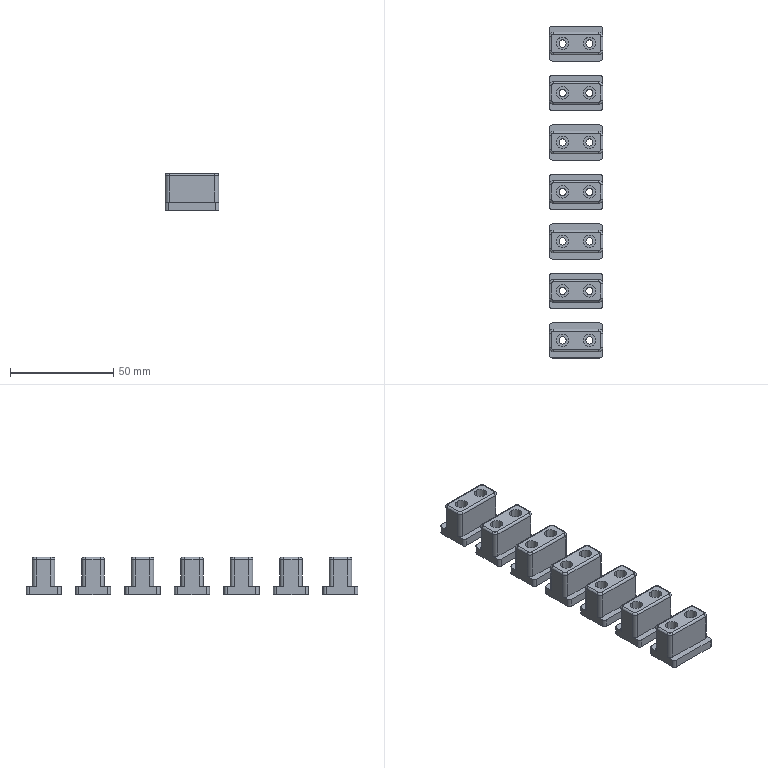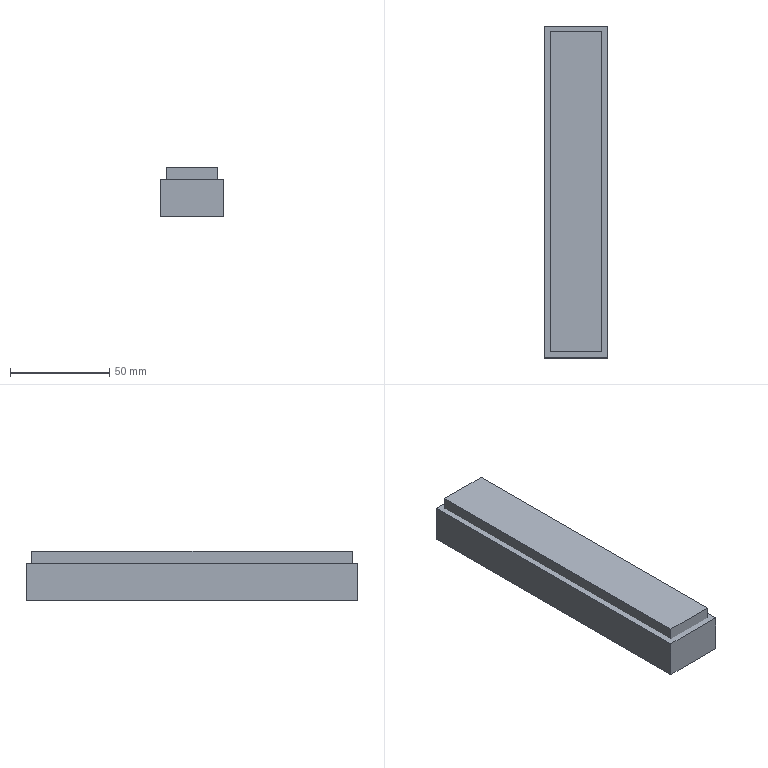CAM job | NX | 3-axis milling, drilling | part box 26 x 161 x 18 mm | stock box 32 x 167 x 25 mm
Tools:
number,name,description,diameter,corner_radius,flute_length,length,flutes
1,D63,Milling Tool-5 Parameters,63.0,0.0,50.0,75.0,2
2,D4A45,Milling Tool-5 Parameters,4.0,0.0,2.0,2.0,2
6,D6,Milling Tool-5 Parameters,6.0,0.0,50.0,75.0,2
15,3.5ZT,Drilling Tool,3.5,0.0,35.0,50.0,2
4,D4,Milling Tool-5 Parameters,4.0,0.0,50.0,75.0,2
8,D6R0.5,Milling Tool-5 Parameters,6.0,0.5,50.0,75.0,2
Operations:
program,operation,operation_type,tool,method,geometry_group,spindle_rpm,surface_speed,feed_per_tooth,feed_cut,feed_plunge,cut_length_mm,path_length_mm,cut_time_min,machine_time_min
1虎钳,FLOOR_WALL,VolumeBased25DMillingOperation,D63,METHOD,A,6500.0,1286.0,0.0962,1250.0,100.0,242.0,296.0,0.1936,0.199
1虎钳,DRILLING_COPY,Operation,D4A45,METHOD,A,5000.0,62.0,0.025,250.0,0.0,50.4,438.312,0.2016,0.2404
1虎钳,DRILLING_COPY_COPY_COPY_COPY_COPY_COPY_1,Operation,3.5ZT,METHOD,A,1910.0,21.0,0.0471,180.0,0.0,329.721,996.955,1.832,1.899
1虎钳,ZLEVEL_PROFILE_COPY_COPY_1_COPY,ZLevelMilling,D6,METHOD,A,9500.0,179.0,0.1158,2200.0,1000.0,26410.747,27188.191,12.151,12.229
1虎钳,ZLEVEL_PROFILE_COPY_COPY_1_COPY_COPY,ZLevelMilling,D6,METHOD,A,9500.0,179.0,0.1158,2200.0,1000.0,18121.593,18803.415,8.383,8.451
1虎钳,ZLEVEL_PROFILE_COPY_COPY_COPY_COPY,ZLevelMilling,D6,MILL_FINISH,A,9500.0,119.0,0.0632,1200.0,1000.0,660.233,1740.145,0.553,0.661
1虎钳,ZLEVEL_PROFILE_COPY_COPY_COPY_COPY_COPY,ZLevelMilling,D6,MILL_FINISH,A,9500.0,119.0,0.0632,1200.0,1000.0,757.314,1854.008,0.6341,0.7438
1虎钳,HOLE_MILLING,CylinderMilling,D4,METHOD,A,9500.0,179.0,0.0789,1500.0,100.0,1564.265,2716.265,1.043,1.158
1虎钳,ZLEVEL_PROFILE_1_COPY_1_COPY_COPY,ZLevelMilling,D4A45,METHOD,A,9500.0,179.0,0.0526,1000.0,100.0,252.781,1363.653,0.2528,0.3639
1虎钳,ZLEVEL_PROFILE_COPY_1_COPY,ZLevelMilling,D6R0.5,METHOD,A,9500.0,179.0,0.1579,3000.0,1000.0,13992.66,14571.309,4.679,4.737
2,FLOOR_WALL_COPY,VolumeBased25DMillingOperation,D63,METHOD,B,6500.0,1286.0,0.0962,1250.0,100.0,1652.0,3368.002,1.322,1.493
2,ZLEVEL_PROFILE_1_COPY_1_COPY_COPY_COPY,ZLevelMilling,D4A45,METHOD,B,9500.0,179.0,0.0526,1000.0,100.0,772.642,2739.007,0.7726,0.9693